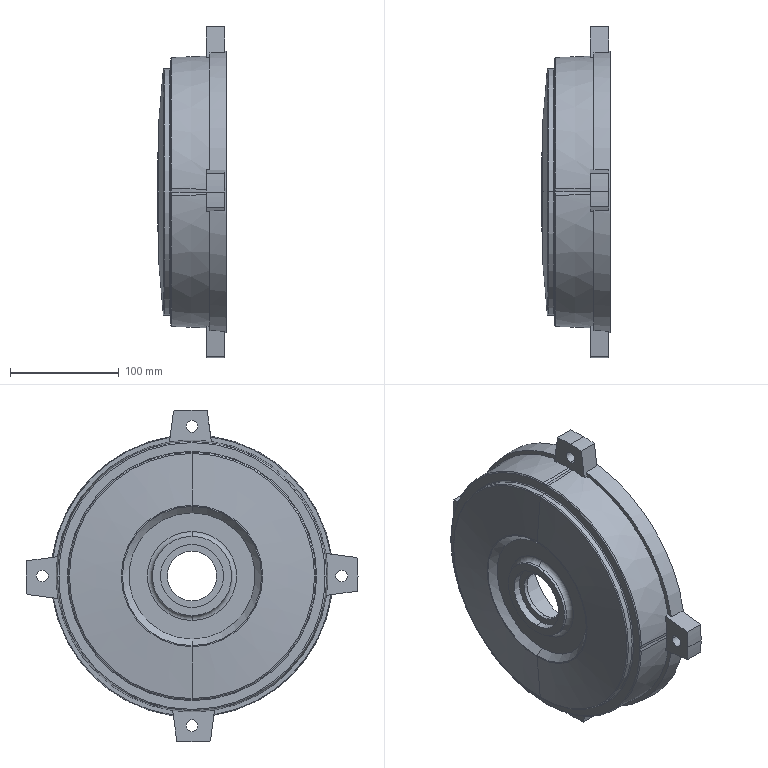Part | STEP file | Input 93 | 1 solid | 112 faces | box 63 x 305 x 305 mm | volume 585521 mm3 | cone 35 | plane 34 | cylinder 30 | torus 13 | commonest cylinder face diameters 11 x8 305 x8 45.5 x2 58 x2 73 x2 90 x2